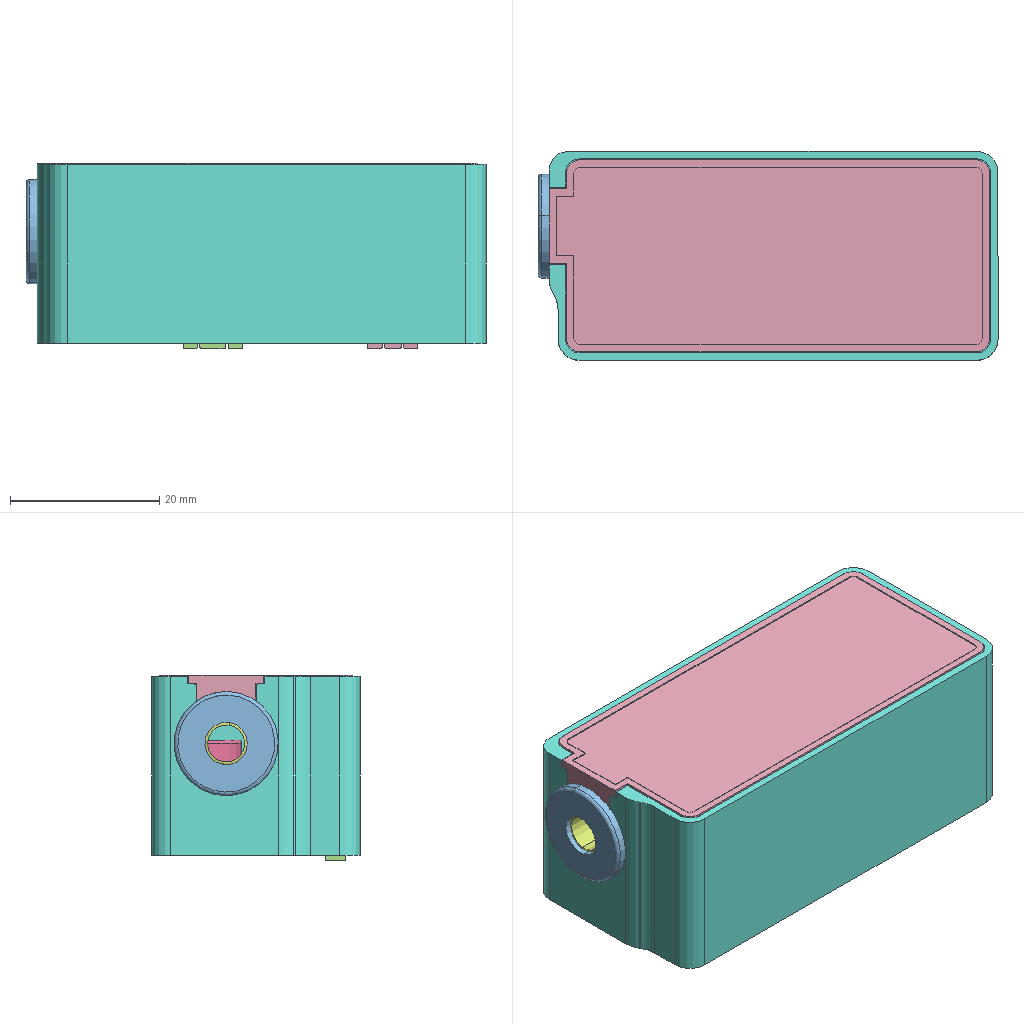Assembly | SolidWorks | 5 different items | 5 placed | box 62 x 28 x 25 mm
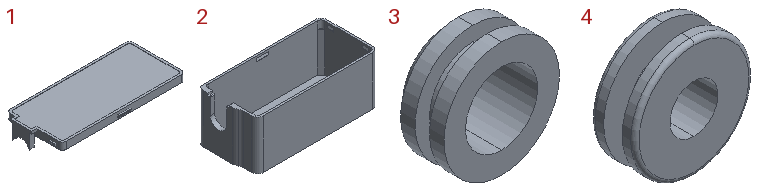Parts list (item | quantity | size | volume | features):
1 | x1 | 59.73 x 27.06 x 7.985 mm | 1980 mm3 | features ICE 12, MirrorSolid 2, Chamfer 1, Cut 1, Extrusion 1, Fillet 1
2 | x1 | 60.2 x 28 x 24 mm | 5859 mm3 | features ICE 9, MirrorPattern 3, Cut 1, DelFace 1, Extrusion 1, Fillet 1
3 | x1 | 8 x 4 x 8 mm | 83.088 mm3 | features Revolution 1
4 | x1 | 14 x 5.2 x 14 mm | 435.063 mm3 | features Revolution 1
5 | x1 | - | - | features BaseBody 182
Mates (type | each side: item.copy, entity, surface, feature):
DistanceDim | 5.1 face plane KH-VM51-BAB-AA-V1.00.step-1/Board.step-1/Open CASCADE STEP translator 7.5 1.1.1.step-1-solid1 | 2.1 face plane Boss-Extrude 2
Width | 5.1 face plane KH-VM51-BAB-AA-V1.00.step-1/Board.step-1/Open CASCADE STEP translator 7.5 1.1.1.step-1-solid1 | 5.1 face plane KH-VM51-BAB-AA-V1.00.step-1/Board.step-1/Open CASCADE STEP translator 7.5 1.1.1.step-1-solid1 | 2.1 face plane Boss-Extrude 1 | 2.1 face plane Boss-Extrude 1 | 2 times
Coincident | 2.1 face plane Boss-Extrude 1 | 1.1 face plane Boss-Extrude 1
Width | 1.1 face plane Boss-Extrude 2 | 1.1 face plane Boss-Extrude 2 | 2.1 face plane Boss-Extrude 1 | 2.1 face plane Boss-Extrude 1 | 2 times
Concentric | 2.1 face cylinder Cut-Extrude 1 | 3.1 face cylinder Revolve 1 | 2 times
Coincident | 2.1 face plane Boss-Extrude 1 | 3.1 face plane Revolve 1
Concentric | 2.1 face cylinder Cut-Extrude 1 | 4.1 face cylinder Revolve 1
Coincident | 2.1 face plane Boss-Extrude 4 | 4.1 face plane Revolve 1